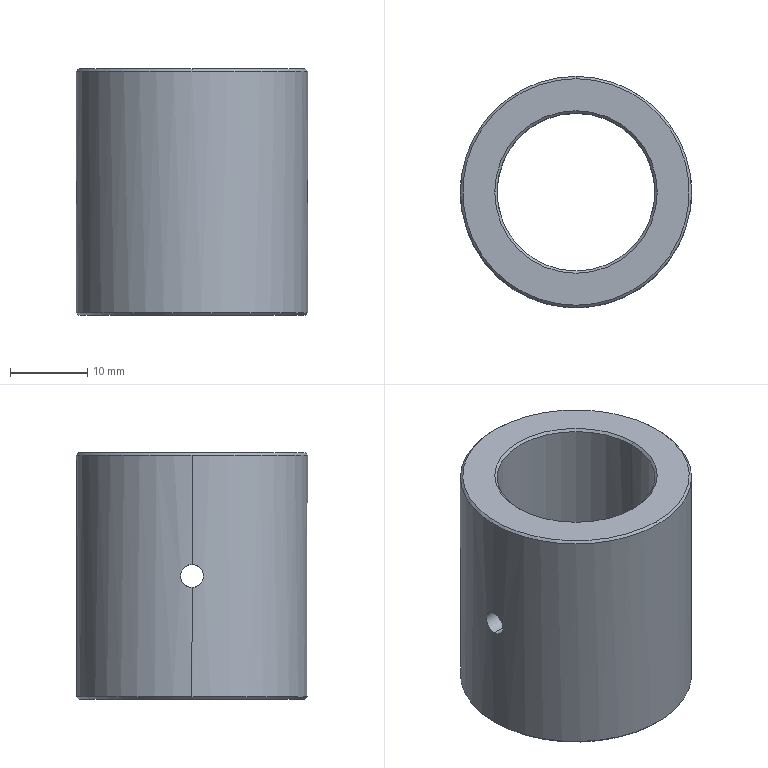Part | STEP file | locating ring 7 | 1 solid | 18 faces | box 30 x 30 x 32 mm | volume 11976 mm3 | cylinder 8 | cone 8 | plane 2 | commonest cylinder face diameters 3 x4 20.5 x2 30 x2